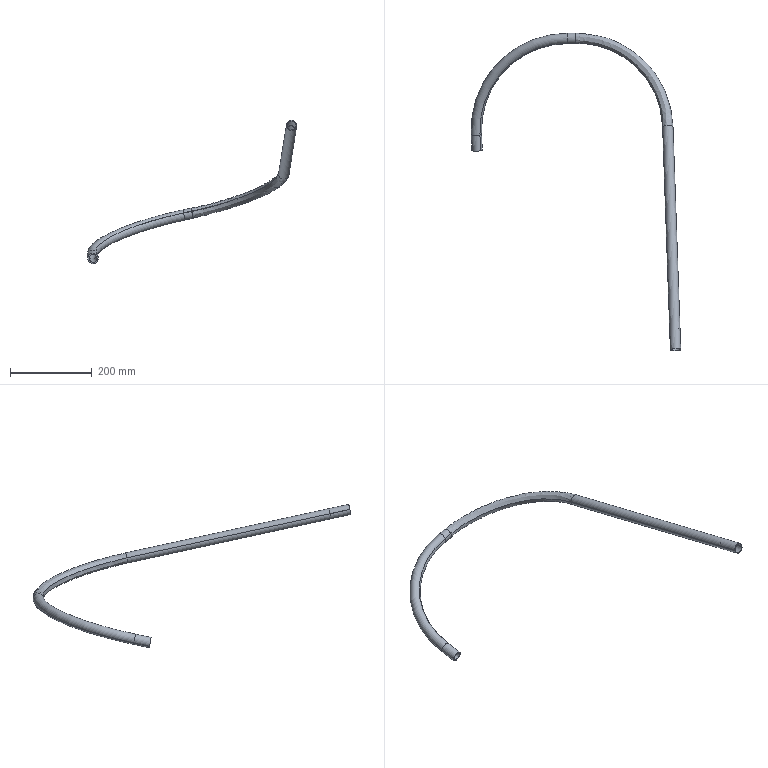Part | STEP file | 31E-01145WG10 | 1 solid | 25 faces | box 512.979 x 777.537 x 350.463 mm | volume 265200 mm3 | cylinder 14 | spline 4 | torus 4 | plane 3 | commonest cylinder face diameters 19.8 x6 25.4 x6 22.2 x2
STEP:
#1=CARTESIAN_POINT('',(-236.061,795.935,-46.108));
#2=VERTEX_POINT('',#1);
#3=CARTESIAN_POINT('',(-20.914,588.327,46.013));
#4=VERTEX_POINT('',#3);
#5=CARTESIAN_POINT('',(-20.914,588.327,46.013));
#6=CARTESIAN_POINT('',(-21.694,610.725,41.15));
#7=CARTESIAN_POINT('',(-25.248,632.89,35.656));
#8=CARTESIAN_POINT('',(-31.561,654.356,29.632));
#9=CARTESIAN_POINT('',(-49.455,695.005,16.849));
#10=CARTESIAN_POINT('',(-76.953,729.545,3.191));
#11=CARTESIAN_POINT('',(-92.871,744.902,-3.704));
#12=CARTESIAN_POINT('',(-128.381,771.151,-17.324));
#13=CARTESIAN_POINT('',(-169.661,787.598,-29.994));
#14=CARTESIAN_POINT('',(-191.348,793.153,-35.944));
#15=CARTESIAN_POINT('',(-213.636,795.932,-41.348));
#16=CARTESIAN_POINT('',(-236.061,795.935,-46.108));
#17=(BOUNDED_CURVE()B_SPLINE_CURVE(5,(#5,#6,#7,#8,#9,#10,#11,#12,#13,#14,#15,#16),.UNSPECIFIED.,.F.,.U.)B_SPLINE_CURVE_WITH_KNOTS((6,3,3,6),(0.,119.553,239.105,358.658),.UNSPECIFIED.)CURVE()GEOMETRIC_REPRESENTATION_ITEM()RATIONAL_B_SPLINE_CURVE((1.,1.,1.,1.,1.,1.,1.,1.,1.,1.,1.,1.))REPRESENTATION_ITEM(''));
#18=EDGE_CURVE('',#2,#4,#17,.F.);
#19=ORIENTED_EDGE('',*,*,#18,.F.);
#20=CARTESIAN_POINT('',(-234.406,814.065,-53.893));
#21=VERTEX_POINT('',#20);
#22=CARTESIAN_POINT('',(-236.061,795.935,-46.108));
#23=CARTESIAN_POINT('',(-237.946,799.915,-37.241));
#24=CARTESIAN_POINT('',(-238.061,810.969,-36.7));
#25=CARTESIAN_POINT('',(-236.291,818.044,-45.026));
#26=CARTESIAN_POINT('',(-234.406,814.065,-53.893));
#27=(BOUNDED_CURVE()B_SPLINE_CURVE(4,(#22,#23,#24,#25,#26),.UNSPECIFIED.,.F.,.U.)B_SPLINE_CURVE_WITH_KNOTS((5,5),(31.029,62.13),.UNSPECIFIED.)CURVE()GEOMETRIC_REPRESENTATION_ITEM()RATIONAL_B_SPLINE_CURVE((1.,0.7071,0.6667,0.7071,1.))REPRESENTATION_ITEM(''));
#28=EDGE_CURVE('',#2,#21,#27,.T.);
#29=ORIENTED_EDGE('',*,*,#28,.T.);
#30=CARTESIAN_POINT('',(-1.126,589.015,46.013));
#31=VERTEX_POINT('',#30);
#32=CARTESIAN_POINT('',(-1.126,589.015,46.013));
#33=CARTESIAN_POINT('',(-1.971,613.287,40.728));
#34=CARTESIAN_POINT('',(-5.823,637.306,34.765));
#35=CARTESIAN_POINT('',(-12.665,660.572,28.234));
#36=CARTESIAN_POINT('',(-32.061,704.635,14.377));
#37=CARTESIAN_POINT('',(-61.872,742.083,-0.4222));
#38=CARTESIAN_POINT('',(-79.13,758.735,-7.894));
#39=CARTESIAN_POINT('',(-117.632,787.197,-22.653));
#40=CARTESIAN_POINT('',(-162.396,805.033,-36.393));
#41=CARTESIAN_POINT('',(-185.915,811.057,-42.848));
#42=CARTESIAN_POINT('',(-210.087,814.068,-48.717));
#43=CARTESIAN_POINT('',(-234.406,814.065,-53.893));
#44=(BOUNDED_CURVE()B_SPLINE_CURVE(5,(#32,#33,#34,#35,#36,#37,#38,#39,#40,#41,#42,#43),.UNSPECIFIED.,.F.,.U.)B_SPLINE_CURVE_WITH_KNOTS((6,3,3,6),(0.,119.553,239.105,358.658),.UNSPECIFIED.)CURVE()GEOMETRIC_REPRESENTATION_ITEM()RATIONAL_B_SPLINE_CURVE((1.,1.,1.,1.,1.,1.,1.,1.,1.,1.,1.,1.))REPRESENTATION_ITEM(''));
#45=EDGE_CURVE('',#21,#31,#44,.F.);
#46=ORIENTED_EDGE('',*,*,#45,.T.);
#47=CARTESIAN_POINT('',(-20.914,588.327,46.013));
#48=CARTESIAN_POINT('',(-20.987,590.428,55.687));
#49=CARTESIAN_POINT('',(-11.13,591.823,60.524));
#50=CARTESIAN_POINT('',(-1.199,591.116,55.687));
#51=CARTESIAN_POINT('',(-1.126,589.015,46.013));
#52=(BOUNDED_CURVE()B_SPLINE_CURVE(4,(#47,#48,#49,#50,#51),.UNSPECIFIED.,.F.,.U.)B_SPLINE_CURVE_WITH_KNOTS((5,5),(31.029,62.13),.UNSPECIFIED.)CURVE()GEOMETRIC_REPRESENTATION_ITEM()RATIONAL_B_SPLINE_CURVE((1.,0.7071,0.6667,0.7071,1.))REPRESENTATION_ITEM(''));
#53=EDGE_CURVE('',#4,#31,#52,.T.);
#54=ORIENTED_EDGE('',*,*,#53,.F.);
#55=EDGE_LOOP('',(#19,#29,#46,#54));
#56=FACE_OUTER_BOUND('',#55,.T.);
#57=CARTESIAN_POINT('',(-20.914,588.327,46.013));
#58=CARTESIAN_POINT('',(-20.987,590.428,55.687));
#59=CARTESIAN_POINT('',(-11.13,591.823,60.524));
#60=CARTESIAN_POINT('',(-1.199,591.116,55.687));
#61=CARTESIAN_POINT('',(-1.126,589.015,46.013));
#62=CARTESIAN_POINT('',(-21.694,610.725,41.15));
#63=CARTESIAN_POINT('',(-21.767,613.043,50.777));
#64=CARTESIAN_POINT('',(-11.943,615.483,55.379));
#65=CARTESIAN_POINT('',(-2.044,615.605,50.355));
#66=CARTESIAN_POINT('',(-1.971,613.287,40.728));
#67=CARTESIAN_POINT('',(-25.248,632.89,35.656));
#68=CARTESIAN_POINT('',(-25.352,635.425,45.229));
#69=CARTESIAN_POINT('',(-15.691,638.9,49.571));
#70=CARTESIAN_POINT('',(-5.927,639.841,44.339));
#71=CARTESIAN_POINT('',(-5.823,637.306,34.765));
#72=CARTESIAN_POINT('',(-31.561,654.356,29.632));
#73=CARTESIAN_POINT('',(-31.725,657.093,39.148));
#74=CARTESIAN_POINT('',(-22.359,661.57,43.207));
#75=CARTESIAN_POINT('',(-12.829,663.309,37.75));
#76=CARTESIAN_POINT('',(-12.665,660.572,28.234));
#77=CARTESIAN_POINT('',(-49.455,695.005,16.849));
#78=CARTESIAN_POINT('',(-49.785,698.116,26.247));
#79=CARTESIAN_POINT('',(-41.252,704.486,29.711));
#80=CARTESIAN_POINT('',(-32.391,707.746,23.776));
#81=CARTESIAN_POINT('',(-32.061,704.635,14.377));
#82=CARTESIAN_POINT('',(-76.953,729.545,3.191));
#83=CARTESIAN_POINT('',(-77.53,732.959,12.469));
#84=CARTESIAN_POINT('',(-70.277,740.935,15.302));
#85=CARTESIAN_POINT('',(-62.449,745.497,8.856));
#86=CARTESIAN_POINT('',(-61.872,742.083,-0.4222));
#87=CARTESIAN_POINT('',(-92.871,744.902,-3.704));
#88=CARTESIAN_POINT('',(-93.588,748.449,5.514));
#89=CARTESIAN_POINT('',(-87.076,757.138,8.028));
#90=CARTESIAN_POINT('',(-79.847,762.281,1.325));
#91=CARTESIAN_POINT('',(-79.13,758.735,-7.894));
#92=CARTESIAN_POINT('',(-128.381,771.151,-17.324));
#93=CARTESIAN_POINT('',(-129.406,774.919,-8.221));
#94=CARTESIAN_POINT('',(-124.544,784.827,-6.335));
#95=CARTESIAN_POINT('',(-118.657,790.966,-13.551));
#96=CARTESIAN_POINT('',(-117.632,787.197,-22.653));
#97=CARTESIAN_POINT('',(-169.661,787.598,-29.994));
#98=CARTESIAN_POINT('',(-171.028,791.501,-20.997));
#99=CARTESIAN_POINT('',(-168.078,802.171,-19.697));
#100=CARTESIAN_POINT('',(-163.762,808.937,-27.395));
#101=CARTESIAN_POINT('',(-162.396,805.033,-36.393));
#102=CARTESIAN_POINT('',(-191.348,793.153,-35.944));
#103=CARTESIAN_POINT('',(-192.888,797.101,-26.994));
#104=CARTESIAN_POINT('',(-190.941,808.027,-25.971));
#105=CARTESIAN_POINT('',(-187.454,815.005,-33.898));
#106=CARTESIAN_POINT('',(-185.915,811.057,-42.848));
#107=CARTESIAN_POINT('',(-213.636,795.932,-41.348));
#108=CARTESIAN_POINT('',(-215.347,799.905,-32.441));
#109=CARTESIAN_POINT('',(-214.428,810.96,-31.672));
#110=CARTESIAN_POINT('',(-211.798,818.041,-39.81));
#111=CARTESIAN_POINT('',(-210.087,814.068,-48.717));
#112=CARTESIAN_POINT('',(-236.061,795.935,-46.108));
#113=CARTESIAN_POINT('',(-237.946,799.915,-37.241));
#114=CARTESIAN_POINT('',(-238.061,810.969,-36.7));
#115=CARTESIAN_POINT('',(-236.291,818.044,-45.026));
#116=CARTESIAN_POINT('',(-234.406,814.065,-53.893));
#117=(BOUNDED_SURFACE()B_SPLINE_SURFACE(5,4,((#57,#58,#59,#60,#61),(#62,#63,#64,#65,#66),(#67,#68,#69,#70,#71),(#72,#73,#74,#75,#76),(#77,#78,#79,#80,#81),(#82,#83,#84,#85,#86),(#87,#88,#89,#90,#91),(#92,#93,#94,#95,#96),(#97,#98,#99,#100,#101),(#102,#103,#104,#105,#106),(#107,#108,#109,#110,#111),(#112,#113,#114,#115,#116)),.UNSPECIFIED.,.F.,.F.,.U.)B_SPLINE_SURFACE_WITH_KNOTS((6,3,3,6),(5,5),(0.,119.553,239.105,358.658),(31.029,62.13),.UNSPECIFIED.)GEOMETRIC_REPRESENTATION_ITEM()RATIONAL_B_SPLINE_SURFACE(((1.,0.7071,0.6667,0.7071,1.),(1.,0.7071,0.6667,0.7071,1.),(1.,0.7071,0.6667,0.7071,1.),(1.,0.7071,0.6667,0.7071,1.),(1.,0.7071,0.6667,0.7071,1.),(1.,0.7071,0.6667,0.7071,1.),(1.,0.7071,0.6667,0.7071,1.),(1.,0.7071,0.6667,0.7071,1.),(1.,0.7071,0.6667,0.7071,1.),(1.,0.7071,0.6667,0.7071,1.),(1.,0.7071,0.6667,0.7071,1.),(1.,0.7071,0.6667,0.7071,1.)))REPRESENTATION_ITEM('')SURFACE());
#118=ADVANCED_FACE('',(#56),#117,.T.);
#119=ORIENTED_EDGE('',*,*,#45,.F.);
#120=CARTESIAN_POINT('',(-234.406,814.065,-53.893));
#121=CARTESIAN_POINT('',(-232.521,810.085,-62.76));
#122=CARTESIAN_POINT('',(-232.406,799.031,-63.301));
#123=CARTESIAN_POINT('',(-234.176,791.956,-54.975));
#124=CARTESIAN_POINT('',(-236.061,795.935,-46.108));
#125=(BOUNDED_CURVE()B_SPLINE_CURVE(4,(#120,#121,#122,#123,#124),.UNSPECIFIED.,.F.,.U.)B_SPLINE_CURVE_WITH_KNOTS((5,5),(62.13,93.232),.UNSPECIFIED.)CURVE()GEOMETRIC_REPRESENTATION_ITEM()RATIONAL_B_SPLINE_CURVE((1.,0.7071,0.6667,0.7071,1.))REPRESENTATION_ITEM(''));
#126=EDGE_CURVE('',#21,#2,#125,.T.);
#127=ORIENTED_EDGE('',*,*,#126,.T.);
#128=ORIENTED_EDGE('',*,*,#18,.T.);
#129=CARTESIAN_POINT('',(-1.126,589.015,46.013));
#130=CARTESIAN_POINT('',(-1.053,586.914,36.338));
#131=CARTESIAN_POINT('',(-10.91,585.52,31.501));
#132=CARTESIAN_POINT('',(-20.841,586.226,36.338));
#133=CARTESIAN_POINT('',(-20.914,588.327,46.013));
#134=(BOUNDED_CURVE()B_SPLINE_CURVE(4,(#129,#130,#131,#132,#133),.UNSPECIFIED.,.F.,.U.)B_SPLINE_CURVE_WITH_KNOTS((5,5),(62.13,93.232),.UNSPECIFIED.)CURVE()GEOMETRIC_REPRESENTATION_ITEM()RATIONAL_B_SPLINE_CURVE((1.,0.7071,0.6667,0.7071,1.))REPRESENTATION_ITEM(''));
#135=EDGE_CURVE('',#31,#4,#134,.T.);
#136=ORIENTED_EDGE('',*,*,#135,.F.);
#137=EDGE_LOOP('',(#119,#127,#128,#136));
#138=FACE_OUTER_BOUND('',#137,.T.);
#139=CARTESIAN_POINT('',(-1.126,589.015,46.013));
#140=CARTESIAN_POINT('',(-1.053,586.914,36.338));
#141=CARTESIAN_POINT('',(-10.91,585.52,31.501));
#142=CARTESIAN_POINT('',(-20.841,586.226,36.338));
#143=CARTESIAN_POINT('',(-20.914,588.327,46.013));
#144=CARTESIAN_POINT('',(-1.971,613.287,40.728));
#145=CARTESIAN_POINT('',(-1.897,610.969,31.101));
#146=CARTESIAN_POINT('',(-11.722,608.529,26.498));
#147=CARTESIAN_POINT('',(-21.62,608.407,31.522));
#148=CARTESIAN_POINT('',(-21.694,610.725,41.15));
#149=CARTESIAN_POINT('',(-5.823,637.306,34.765));
#150=CARTESIAN_POINT('',(-5.719,634.772,25.192));
#151=CARTESIAN_POINT('',(-15.38,631.297,20.85));
#152=CARTESIAN_POINT('',(-25.144,630.356,26.082));
#153=CARTESIAN_POINT('',(-25.248,632.89,35.656));
#154=CARTESIAN_POINT('',(-12.665,660.572,28.234));
#155=CARTESIAN_POINT('',(-12.502,657.834,18.718));
#156=CARTESIAN_POINT('',(-21.868,653.358,14.659));
#157=CARTESIAN_POINT('',(-31.398,651.619,20.116));
#158=CARTESIAN_POINT('',(-31.561,654.356,29.632));
#159=CARTESIAN_POINT('',(-32.061,704.635,14.377));
#160=CARTESIAN_POINT('',(-31.732,701.524,4.979));
#161=CARTESIAN_POINT('',(-40.265,695.154,1.515));
#162=CARTESIAN_POINT('',(-49.126,691.894,7.45));
#163=CARTESIAN_POINT('',(-49.455,695.005,16.849));
#164=CARTESIAN_POINT('',(-61.872,742.083,-0.4222));
#165=CARTESIAN_POINT('',(-61.296,738.669,-9.7));
#166=CARTESIAN_POINT('',(-68.548,730.693,-12.533));
#167=CARTESIAN_POINT('',(-76.377,726.131,-6.087));
#168=CARTESIAN_POINT('',(-76.953,729.545,3.191));
#169=CARTESIAN_POINT('',(-79.13,758.735,-7.894));
#170=CARTESIAN_POINT('',(-78.413,755.188,-17.112));
#171=CARTESIAN_POINT('',(-84.925,746.499,-19.627));
#172=CARTESIAN_POINT('',(-92.154,741.356,-12.923));
#173=CARTESIAN_POINT('',(-92.871,744.902,-3.704));
#174=CARTESIAN_POINT('',(-117.632,787.197,-22.653));
#175=CARTESIAN_POINT('',(-116.607,783.429,-31.756));
#176=CARTESIAN_POINT('',(-121.468,773.521,-33.642));
#177=CARTESIAN_POINT('',(-127.356,767.382,-26.426));
#178=CARTESIAN_POINT('',(-128.381,771.151,-17.324));
#179=CARTESIAN_POINT('',(-162.396,805.033,-36.393));
#180=CARTESIAN_POINT('',(-161.029,801.13,-45.391));
#181=CARTESIAN_POINT('',(-163.979,790.461,-46.691));
#182=CARTESIAN_POINT('',(-168.295,783.695,-38.992));
#183=CARTESIAN_POINT('',(-169.661,787.598,-29.994));
#184=CARTESIAN_POINT('',(-185.915,811.057,-42.848));
#185=CARTESIAN_POINT('',(-184.375,807.11,-51.798));
#186=CARTESIAN_POINT('',(-186.321,796.184,-52.821));
#187=CARTESIAN_POINT('',(-189.808,789.206,-44.894));
#188=CARTESIAN_POINT('',(-191.348,793.153,-35.944));
#189=CARTESIAN_POINT('',(-210.087,814.068,-48.717));
#190=CARTESIAN_POINT('',(-208.376,810.095,-57.624));
#191=CARTESIAN_POINT('',(-209.295,799.04,-58.393));
#192=CARTESIAN_POINT('',(-211.925,791.959,-50.255));
#193=CARTESIAN_POINT('',(-213.636,795.932,-41.348));
#194=CARTESIAN_POINT('',(-234.406,814.065,-53.893));
#195=CARTESIAN_POINT('',(-232.521,810.085,-62.76));
#196=CARTESIAN_POINT('',(-232.406,799.031,-63.301));
#197=CARTESIAN_POINT('',(-234.176,791.956,-54.975));
#198=CARTESIAN_POINT('',(-236.061,795.935,-46.108));
#199=(BOUNDED_SURFACE()B_SPLINE_SURFACE(5,4,((#139,#140,#141,#142,#143),(#144,#145,#146,#147,#148),(#149,#150,#151,#152,#153),(#154,#155,#156,#157,#158),(#159,#160,#161,#162,#163),(#164,#165,#166,#167,#168),(#169,#170,#171,#172,#173),(#174,#175,#176,#177,#178),(#179,#180,#181,#182,#183),(#184,#185,#186,#187,#188),(#189,#190,#191,#192,#193),(#194,#195,#196,#197,#198)),.UNSPECIFIED.,.F.,.F.,.U.)B_SPLINE_SURFACE_WITH_KNOTS((6,3,3,6),(5,5),(0.,119.553,239.105,358.658),(62.13,93.232),.UNSPECIFIED.)GEOMETRIC_REPRESENTATION_ITEM()RATIONAL_B_SPLINE_SURFACE(((1.,0.7071,0.6667,0.7071,1.),(1.,0.7071,0.6667,0.7071,1.),(1.,0.7071,0.6667,0.7071,1.),(1.,0.7071,0.6667,0.7071,1.),(1.,0.7071,0.6667,0.7071,1.),(1.,0.7071,0.6667,0.7071,1.),(1.,0.7071,0.6667,0.7071,1.),(1.,0.7071,0.6667,0.7071,1.),(1.,0.7071,0.6667,0.7071,1.),(1.,0.7071,0.6667,0.7071,1.),(1.,0.7071,0.6667,0.7071,1.),(1.,0.7071,0.6667,0.7071,1.)))REPRESENTATION_ITEM('')SURFACE());
#200=ADVANCED_FACE('',(#138),#199,.T.);
#201=CARTESIAN_POINT('',(20.666,43.336,164.685));
#202=VERTEX_POINT('',#201);
#203=CARTESIAN_POINT('',(1.672,589.113,46.013));
#204=VERTEX_POINT('',#203);
#205=CARTESIAN_POINT('',(11.169,316.224,105.349));
#206=DIRECTION('',(-0.03399,0.9766,-0.2123));
#207=VECTOR('',#206,1.);
#208=LINE('',#205,#207);
#209=EDGE_CURVE('',#202,#204,#208,.T.);
#210=ORIENTED_EDGE('',*,*,#209,.F.);
#211=CARTESIAN_POINT('',(-4.719,42.452,164.685));
#212=VERTEX_POINT('',#211);
#213=CARTESIAN_POINT('',(7.974,42.894,164.685));
#214=DIRECTION('',(-0.03399,0.9766,-0.2123));
#215=AXIS2_PLACEMENT_3D('',#213,#214,$);
#216=CIRCLE('',#215,12.7);
#217=EDGE_CURVE('',#202,#212,#216,.T.);
#218=ORIENTED_EDGE('',*,*,#217,.T.);
#219=CARTESIAN_POINT('',(-23.712,588.229,46.013));
#220=VERTEX_POINT('',#219);
#221=CARTESIAN_POINT('',(-14.215,315.341,105.349));
#222=DIRECTION('',(-0.03399,0.9766,-0.2123));
#223=VECTOR('',#222,1.);
#224=LINE('',#221,#223);
#225=EDGE_CURVE('',#212,#220,#224,.T.);
#226=ORIENTED_EDGE('',*,*,#225,.T.);
#227=CARTESIAN_POINT('',(-11.02,588.671,46.013));
#228=DIRECTION('',(-0.03399,0.9766,-0.2123));
#229=AXIS2_PLACEMENT_3D('',#227,#228,$);
#230=CIRCLE('',#229,12.7);
#231=EDGE_CURVE('',#204,#220,#230,.T.);
#232=ORIENTED_EDGE('',*,*,#231,.F.);
#233=EDGE_LOOP('',(#210,#218,#226,#232));
#234=FACE_OUTER_BOUND('',#233,.T.);
#235=CARTESIAN_POINT('',(-1.523,315.782,105.349));
#236=DIRECTION('',(-0.03399,0.9766,-0.2123));
#237=DIRECTION('',(0.9994,0.03478,0.));
#238=AXIS2_PLACEMENT_3D('',#235,#236,#237);
#239=CYLINDRICAL_SURFACE('',#238,12.7);
#240=ADVANCED_FACE('',(#234),#239,.T.);
#241=ORIENTED_EDGE('',*,*,#225,.F.);
#242=CARTESIAN_POINT('',(7.974,42.894,164.685));
#243=DIRECTION('',(-0.03399,0.9766,-0.2123));
#244=AXIS2_PLACEMENT_3D('',#242,#243,$);
#245=CIRCLE('',#244,12.7);
#246=EDGE_CURVE('',#212,#202,#245,.T.);
#247=ORIENTED_EDGE('',*,*,#246,.T.);
#248=ORIENTED_EDGE('',*,*,#209,.T.);
#249=CARTESIAN_POINT('',(-11.02,588.671,46.013));
#250=DIRECTION('',(-0.03399,0.9766,-0.2123));
#251=AXIS2_PLACEMENT_3D('',#249,#250,$);
#252=CIRCLE('',#251,12.7);
#253=EDGE_CURVE('',#220,#204,#252,.T.);
#254=ORIENTED_EDGE('',*,*,#253,.F.);
#255=EDGE_LOOP('',(#241,#247,#248,#254));
#256=FACE_OUTER_BOUND('',#255,.T.);
#257=CARTESIAN_POINT('',(-1.523,315.782,105.349));
#258=DIRECTION('',(-0.03399,0.9766,-0.2123));
#259=DIRECTION('',(-0.9994,-0.03478,0.));
#260=AXIS2_PLACEMENT_3D('',#257,#258,#259);
#261=CYLINDRICAL_SURFACE('',#260,12.7);
#262=ADVANCED_FACE('',(#256),#261,.T.);
#263=CARTESIAN_POINT('',(-255.83,795.935,-50.31));
#264=VERTEX_POINT('',#263);
#265=CARTESIAN_POINT('',(-254.176,814.065,-58.095));
#266=VERTEX_POINT('',#265);
#267=CARTESIAN_POINT('',(-255.003,805.,-54.203));
#268=DIRECTION('',(-0.9781,0.,-0.2079));
#269=AXIS2_PLACEMENT_3D('',#267,#268,$);
#270=CIRCLE('',#269,9.9);
#271=EDGE_CURVE('',#264,#266,#270,.T.);
#272=ORIENTED_EDGE('',*,*,#271,.T.);
#273=CARTESIAN_POINT('',(-244.291,814.065,-55.994));
#274=DIRECTION('',(-0.9781,0.,-0.2079));
#275=VECTOR('',#274,1.);
#276=LINE('',#273,#275);
#277=EDGE_CURVE('',#21,#266,#276,.T.);
#278=ORIENTED_EDGE('',*,*,#277,.F.);
#279=ORIENTED_EDGE('',*,*,#28,.F.);
#280=CARTESIAN_POINT('',(-245.946,795.935,-48.209));
#281=DIRECTION('',(-0.9781,0.,-0.2079));
#282=VECTOR('',#281,1.);
#283=LINE('',#280,#282);
#284=EDGE_CURVE('',#2,#264,#283,.T.);
#285=ORIENTED_EDGE('',*,*,#284,.T.);
#286=EDGE_LOOP('',(#272,#278,#279,#285));
#287=FACE_OUTER_BOUND('',#286,.T.);
#288=CARTESIAN_POINT('',(-245.118,805.,-52.101));
#289=DIRECTION('',(-0.9781,0.,-0.2079));
#290=DIRECTION('',(-0.08357,-0.9157,0.3932));
#291=AXIS2_PLACEMENT_3D('',#288,#289,#290);
#292=CYLINDRICAL_SURFACE('',#291,9.9);
#293=ADVANCED_FACE('',(#287),#292,.F.);
#294=CARTESIAN_POINT('',(-255.003,805.,-54.203));
#295=DIRECTION('',(-0.9781,0.,-0.2079));
#296=AXIS2_PLACEMENT_3D('',#294,#295,$);
#297=CIRCLE('',#296,9.9);
#298=EDGE_CURVE('',#266,#264,#297,.T.);
#299=ORIENTED_EDGE('',*,*,#298,.T.);
#300=ORIENTED_EDGE('',*,*,#284,.F.);
#301=ORIENTED_EDGE('',*,*,#126,.F.);
#302=ORIENTED_EDGE('',*,*,#277,.T.);
#303=EDGE_LOOP('',(#299,#300,#301,#302));
#304=FACE_OUTER_BOUND('',#303,.T.);
#305=CARTESIAN_POINT('',(-245.118,805.,-52.101));
#306=DIRECTION('',(-0.9781,0.,-0.2079));
#307=DIRECTION('',(0.08357,0.9157,-0.3932));
#308=AXIS2_PLACEMENT_3D('',#305,#306,#307);
#309=CYLINDRICAL_SURFACE('',#308,9.9);
#310=ADVANCED_FACE('',(#304),#309,.F.);
#311=ORIENTED_EDGE('',*,*,#231,.T.);
#312=CARTESIAN_POINT('',(-236.295,793.371,-45.007));
#313=VERTEX_POINT('',#312);
#314=CARTESIAN_POINT('',(-23.712,588.229,46.013));
#315=CARTESIAN_POINT('',(-24.483,610.363,41.209));
#316=CARTESIAN_POINT('',(-27.995,632.266,35.782));
#317=CARTESIAN_POINT('',(-34.234,653.477,29.83));
#318=CARTESIAN_POINT('',(-51.915,693.644,17.198));
#319=CARTESIAN_POINT('',(-79.086,727.772,3.702));
#320=CARTESIAN_POINT('',(-94.814,742.946,-3.112));
#321=CARTESIAN_POINT('',(-129.901,768.881,-16.57));
#322=CARTESIAN_POINT('',(-170.689,785.133,-29.09));
#323=CARTESIAN_POINT('',(-192.116,790.621,-34.968));
#324=CARTESIAN_POINT('',(-214.138,793.368,-40.306));
#325=CARTESIAN_POINT('',(-236.295,793.371,-45.007));
#326=(BOUNDED_CURVE()B_SPLINE_CURVE(5,(#314,#315,#316,#317,#318,#319,#320,#321,#322,#323,#324,#325),.UNSPECIFIED.,.F.,.U.)B_SPLINE_CURVE_WITH_KNOTS((6,3,3,6),(0.,119.604,239.209,358.815),.UNSPECIFIED.)CURVE()GEOMETRIC_REPRESENTATION_ITEM()RATIONAL_B_SPLINE_CURVE((1.,1.,1.,1.,1.,1.,1.,1.,1.,1.,1.,1.))REPRESENTATION_ITEM(''));
#327=EDGE_CURVE('',#313,#220,#326,.F.);
#328=ORIENTED_EDGE('',*,*,#327,.F.);
#329=CARTESIAN_POINT('',(-234.172,816.629,-54.994));
#330=VERTEX_POINT('',#329);
#331=CARTESIAN_POINT('',(-234.172,816.629,-54.994));
#332=CARTESIAN_POINT('',(-231.754,811.524,-66.369));
#333=CARTESIAN_POINT('',(-231.607,797.342,-67.062));
#334=CARTESIAN_POINT('',(-233.877,788.266,-56.382));
#335=CARTESIAN_POINT('',(-236.295,793.371,-45.007));
#336=(BOUNDED_CURVE()B_SPLINE_CURVE(4,(#331,#332,#333,#334,#335),.UNSPECIFIED.,.F.,.U.)B_SPLINE_CURVE_WITH_KNOTS((5,5),(79.703,119.601),.UNSPECIFIED.)CURVE()GEOMETRIC_REPRESENTATION_ITEM()RATIONAL_B_SPLINE_CURVE((1.,0.7071,0.6667,0.7071,1.))REPRESENTATION_ITEM(''));
#337=EDGE_CURVE('',#330,#313,#336,.T.);
#338=ORIENTED_EDGE('',*,*,#337,.F.);
#339=CARTESIAN_POINT('',(1.672,589.113,46.013));
#340=CARTESIAN_POINT('',(0.8184,613.649,40.668));
#341=CARTESIAN_POINT('',(-3.076,637.93,34.64));
#342=CARTESIAN_POINT('',(-9.993,661.451,28.036));
#343=CARTESIAN_POINT('',(-29.602,705.997,14.028));
#344=CARTESIAN_POINT('',(-59.74,743.856,-0.9331));
#345=CARTESIAN_POINT('',(-77.187,760.691,-8.486));
#346=CARTESIAN_POINT('',(-116.112,789.467,-23.407));
#347=CARTESIAN_POINT('',(-161.368,807.499,-37.298));
#348=CARTESIAN_POINT('',(-185.146,813.589,-43.824));
#349=CARTESIAN_POINT('',(-209.585,816.632,-49.759));
#350=CARTESIAN_POINT('',(-234.172,816.629,-54.994));
#351=(BOUNDED_CURVE()B_SPLINE_CURVE(5,(#339,#340,#341,#342,#343,#344,#345,#346,#347,#348,#349,#350),.UNSPECIFIED.,.F.,.U.)B_SPLINE_CURVE_WITH_KNOTS((6,3,3,6),(0.,119.604,239.209,358.815),.UNSPECIFIED.)CURVE()GEOMETRIC_REPRESENTATION_ITEM()RATIONAL_B_SPLINE_CURVE((1.,1.,1.,1.,1.,1.,1.,1.,1.,1.,1.,1.))REPRESENTATION_ITEM(''));
#352=EDGE_CURVE('',#330,#204,#351,.F.);
#353=ORIENTED_EDGE('',*,*,#352,.T.);
#354=EDGE_LOOP('',(#311,#328,#338,#353));
#355=FACE_OUTER_BOUND('',#354,.T.);
#356=CARTESIAN_POINT('',(1.672,589.113,46.013));
#357=CARTESIAN_POINT('',(1.766,586.418,33.602));
#358=CARTESIAN_POINT('',(-10.879,584.628,27.397));
#359=CARTESIAN_POINT('',(-23.619,585.534,33.602));
#360=CARTESIAN_POINT('',(-23.712,588.229,46.013));
#361=CARTESIAN_POINT('',(0.8184,613.649,40.668));
#362=CARTESIAN_POINT('',(0.9129,610.676,28.318));
#363=CARTESIAN_POINT('',(-11.69,607.546,22.414));
#364=CARTESIAN_POINT('',(-24.388,607.389,28.859));
#365=CARTESIAN_POINT('',(-24.483,610.363,41.209));
#366=CARTESIAN_POINT('',(-3.076,637.93,34.64));
#367=CARTESIAN_POINT('',(-2.943,634.679,22.358));
#368=CARTESIAN_POINT('',(-15.336,630.221,16.789));
#369=CARTESIAN_POINT('',(-27.862,629.014,23.501));
#370=CARTESIAN_POINT('',(-27.995,632.266,35.782));
#371=CARTESIAN_POINT('',(-9.993,661.451,28.036));
#372=CARTESIAN_POINT('',(-9.783,657.939,15.828));
#373=CARTESIAN_POINT('',(-21.799,652.197,10.621));
#374=CARTESIAN_POINT('',(-34.024,649.966,17.622));
#375=CARTESIAN_POINT('',(-34.234,653.477,29.83));
#376=CARTESIAN_POINT('',(-29.602,705.997,14.028));
#377=CARTESIAN_POINT('',(-29.18,702.006,1.971));
#378=CARTESIAN_POINT('',(-40.125,693.834,-2.472));
#379=CARTESIAN_POINT('',(-51.493,689.653,5.141));
#380=CARTESIAN_POINT('',(-51.915,693.644,17.198));
#381=CARTESIAN_POINT('',(-59.74,743.856,-0.9331));
#382=CARTESIAN_POINT('',(-59.,739.477,-12.835));
#383=CARTESIAN_POINT('',(-68.303,729.245,-16.469));
#384=CARTESIAN_POINT('',(-78.346,723.393,-8.2));
#385=CARTESIAN_POINT('',(-79.086,727.772,3.702));
#386=CARTESIAN_POINT('',(-77.187,760.691,-8.486));
#387=CARTESIAN_POINT('',(-76.267,756.141,-20.312));
#388=CARTESIAN_POINT('',(-84.621,744.994,-23.537));
#389=CARTESIAN_POINT('',(-93.894,738.397,-14.937));
#390=CARTESIAN_POINT('',(-94.814,742.946,-3.112));
#391=CARTESIAN_POINT('',(-116.112,789.467,-23.407));
#392=CARTESIAN_POINT('',(-114.797,784.632,-35.084));
#393=CARTESIAN_POINT('',(-121.034,771.922,-37.503));
#394=CARTESIAN_POINT('',(-128.586,764.047,-28.246));
#395=CARTESIAN_POINT('',(-129.901,768.881,-16.57));
#396=CARTESIAN_POINT('',(-161.368,807.499,-37.298));
#397=CARTESIAN_POINT('',(-159.615,802.492,-48.841));
#398=CARTESIAN_POINT('',(-163.399,788.805,-50.508));
#399=CARTESIAN_POINT('',(-168.936,780.125,-40.632));
#400=CARTESIAN_POINT('',(-170.689,785.133,-29.09));
#401=CARTESIAN_POINT('',(-185.146,813.589,-43.824));
#402=CARTESIAN_POINT('',(-183.171,808.525,-55.306));
#403=CARTESIAN_POINT('',(-185.668,794.509,-56.618));
#404=CARTESIAN_POINT('',(-190.141,785.557,-46.449));
#405=CARTESIAN_POINT('',(-192.116,790.621,-34.968));
#406=CARTESIAN_POINT('',(-209.585,816.632,-49.759));
#407=CARTESIAN_POINT('',(-207.39,811.536,-61.185));
#408=CARTESIAN_POINT('',(-208.569,797.355,-62.171));
#409=CARTESIAN_POINT('',(-211.943,788.271,-51.731));
#410=CARTESIAN_POINT('',(-214.138,793.368,-40.306));
#411=CARTESIAN_POINT('',(-234.172,816.629,-54.994));
#412=CARTESIAN_POINT('',(-231.754,811.524,-66.369));
#413=CARTESIAN_POINT('',(-231.607,797.342,-67.062));
#414=CARTESIAN_POINT('',(-233.877,788.266,-56.382));
#415=CARTESIAN_POINT('',(-236.295,793.371,-45.007));
#416=(BOUNDED_SURFACE()B_SPLINE_SURFACE(5,4,((#356,#357,#358,#359,#360),(#361,#362,#363,#364,#365),(#366,#367,#368,#369,#370),(#371,#372,#373,#374,#375),(#376,#377,#378,#379,#380),(#381,#382,#383,#384,#385),(#386,#387,#388,#389,#390),(#391,#392,#393,#394,#395),(#396,#397,#398,#399,#400),(#401,#402,#403,#404,#405),(#406,#407,#408,#409,#410),(#411,#412,#413,#414,#415)),.UNSPECIFIED.,.F.,.F.,.U.)B_SPLINE_SURFACE_WITH_KNOTS((6,3,3,6),(5,5),(0.,119.604,239.209,358.815),(79.703,119.601),.UNSPECIFIED.)GEOMETRIC_REPRESENTATION_ITEM()RATIONAL_B_SPLINE_SURFACE(((1.,0.7071,0.6667,0.7071,1.),(1.,0.7071,0.6667,0.7071,1.),(1.,0.7071,0.6667,0.7071,1.),(1.,0.7071,0.6667,0.7071,1.),(1.,0.7071,0.6667,0.7071,1.),(1.,0.7071,0.6667,0.7071,1.),(1.,0.7071,0.6667,0.7071,1.),(1.,0.7071,0.6667,0.7071,1.),(1.,0.7071,0.6667,0.7071,1.),(1.,0.7071,0.6667,0.7071,1.),(1.,0.7071,0.6667,0.7071,1.),(1.,0.7071,0.6667,0.7071,1.)))REPRESENTATION_ITEM('')SURFACE());
#417=ADVANCED_FACE('',(#355),#416,.F.);
#418=ORIENTED_EDGE('',*,*,#253,.T.);
#419=ORIENTED_EDGE('',*,*,#352,.F.);
#420=CARTESIAN_POINT('',(-236.295,793.371,-45.007));
#421=CARTESIAN_POINT('',(-238.713,798.476,-33.632));
#422=CARTESIAN_POINT('',(-238.86,812.658,-32.938));
#423=CARTESIAN_POINT('',(-236.59,821.734,-43.619));
#424=CARTESIAN_POINT('',(-234.172,816.629,-54.994));
#425=(BOUNDED_CURVE()B_SPLINE_CURVE(4,(#420,#421,#422,#423,#424),.UNSPECIFIED.,.F.,.U.)B_SPLINE_CURVE_WITH_KNOTS((5,5),(39.804,79.703),.UNSPECIFIED.)CURVE()GEOMETRIC_REPRESENTATION_ITEM()RATIONAL_B_SPLINE_CURVE((1.,0.7071,0.6667,0.7071,1.))REPRESENTATION_ITEM(''));
#426=EDGE_CURVE('',#313,#330,#425,.T.);
#427=ORIENTED_EDGE('',*,*,#426,.F.);
#428=ORIENTED_EDGE('',*,*,#327,.T.);
#429=EDGE_LOOP('',(#418,#419,#427,#428));
#430=FACE_OUTER_BOUND('',#429,.T.);
#431=CARTESIAN_POINT('',(-23.712,588.229,46.013));
#432=CARTESIAN_POINT('',(-23.806,590.925,58.423));
#433=CARTESIAN_POINT('',(-11.161,592.714,64.628));
#434=CARTESIAN_POINT('',(1.579,591.808,58.423));
#435=CARTESIAN_POINT('',(1.672,589.113,46.013));
#436=CARTESIAN_POINT('',(-24.483,610.363,41.209));
#437=CARTESIAN_POINT('',(-24.577,613.336,53.559));
#438=CARTESIAN_POINT('',(-11.974,616.466,59.464));
#439=CARTESIAN_POINT('',(0.724,616.623,53.018));
#440=CARTESIAN_POINT('',(0.8184,613.649,40.668));
#441=CARTESIAN_POINT('',(-27.995,632.266,35.782));
#442=CARTESIAN_POINT('',(-28.128,635.517,48.063));
#443=CARTESIAN_POINT('',(-15.735,639.975,53.632));
#444=CARTESIAN_POINT('',(-3.209,641.182,46.921));
#445=CARTESIAN_POINT('',(-3.076,637.93,34.64));
#446=CARTESIAN_POINT('',(-34.234,653.477,29.83));
#447=CARTESIAN_POINT('',(-34.444,656.989,42.037));
#448=CARTESIAN_POINT('',(-22.428,662.732,47.244));
#449=CARTESIAN_POINT('',(-10.203,664.963,40.244));
#450=CARTESIAN_POINT('',(-9.993,661.451,28.036));
#451=CARTESIAN_POINT('',(-51.915,693.644,17.198));
#452=CARTESIAN_POINT('',(-52.338,697.634,29.255));
#453=CARTESIAN_POINT('',(-41.392,705.806,33.698));
#454=CARTESIAN_POINT('',(-30.024,709.987,26.084));
#455=CARTESIAN_POINT('',(-29.602,705.997,14.028));
#456=CARTESIAN_POINT('',(-79.086,727.772,3.702));
#457=CARTESIAN_POINT('',(-79.825,732.152,15.604));
#458=CARTESIAN_POINT('',(-70.522,742.384,19.238));
#459=CARTESIAN_POINT('',(-60.479,748.236,10.969));
#460=CARTESIAN_POINT('',(-59.74,743.856,-0.9331));
#461=CARTESIAN_POINT('',(-94.814,742.946,-3.112));
#462=CARTESIAN_POINT('',(-95.734,747.495,8.714));
#463=CARTESIAN_POINT('',(-87.38,758.642,11.939));
#464=CARTESIAN_POINT('',(-78.107,765.24,3.339));
#465=CARTESIAN_POINT('',(-77.187,760.691,-8.486));
#466=CARTESIAN_POINT('',(-129.901,768.881,-16.57));
#467=CARTESIAN_POINT('',(-131.216,773.716,-4.893));
#468=CARTESIAN_POINT('',(-124.979,786.426,-2.474));
#469=CARTESIAN_POINT('',(-117.427,794.301,-11.73));
#470=CARTESIAN_POINT('',(-116.112,789.467,-23.407));
#471=CARTESIAN_POINT('',(-170.689,785.133,-29.09));
#472=CARTESIAN_POINT('',(-172.442,790.14,-17.547));
#473=CARTESIAN_POINT('',(-168.658,803.827,-15.88));
#474=CARTESIAN_POINT('',(-163.121,812.506,-25.755));
#475=CARTESIAN_POINT('',(-161.368,807.499,-37.298));
#476=CARTESIAN_POINT('',(-192.116,790.621,-34.968));
#477=CARTESIAN_POINT('',(-194.092,795.685,-23.486));
#478=CARTESIAN_POINT('',(-191.594,809.701,-22.174));
#479=CARTESIAN_POINT('',(-187.122,818.653,-32.343));
#480=CARTESIAN_POINT('',(-185.146,813.589,-43.824));
#481=CARTESIAN_POINT('',(-214.138,793.368,-40.306));
#482=CARTESIAN_POINT('',(-216.332,798.464,-28.88));
#483=CARTESIAN_POINT('',(-215.154,812.645,-27.894));
#484=CARTESIAN_POINT('',(-211.78,821.729,-38.334));
#485=CARTESIAN_POINT('',(-209.585,816.632,-49.759));
#486=CARTESIAN_POINT('',(-236.295,793.371,-45.007));
#487=CARTESIAN_POINT('',(-238.713,798.476,-33.632));
#488=CARTESIAN_POINT('',(-238.86,812.658,-32.938));
#489=CARTESIAN_POINT('',(-236.59,821.734,-43.619));
#490=CARTESIAN_POINT('',(-234.172,816.629,-54.994));
#491=(BOUNDED_SURFACE()B_SPLINE_SURFACE(5,4,((#431,#432,#433,#434,#435),(#436,#437,#438,#439,#440),(#441,#442,#443,#444,#445),(#446,#447,#448,#449,#450),(#451,#452,#453,#454,#455),(#456,#457,#458,#459,#460),(#461,#462,#463,#464,#465),(#466,#467,#468,#469,#470),(#471,#472,#473,#474,#475),(#476,#477,#478,#479,#480),(#481,#482,#483,#484,#485),(#486,#487,#488,#489,#490)),.UNSPECIFIED.,.F.,.F.,.U.)B_SPLINE_SURFACE_WITH_KNOTS((6,3,3,6),(5,5),(0.,119.604,239.209,358.815),(39.804,79.703),.UNSPECIFIED.)GEOMETRIC_REPRESENTATION_ITEM()RATIONAL_B_SPLINE_SURFACE(((1.,0.7071,0.6667,0.7071,1.),(1.,0.7071,0.6667,0.7071,1.),(1.,0.7071,0.6667,0.7071,1.),(1.,0.7071,0.6667,0.7071,1.),(1.,0.7071,0.6667,0.7071,1.),(1.,0.7071,0.6667,0.7071,1.),(1.,0.7071,0.6667,0.7071,1.),(1.,0.7071,0.6667,0.7071,1.),(1.,0.7071,0.6667,0.7071,1.),(1.,0.7071,0.6667,0.7071,1.),(1.,0.7071,0.6667,0.7071,1.),(1.,0.7071,0.6667,0.7071,1.)))REPRESENTATION_ITEM('')SURFACE());
#492=ADVANCED_FACE('',(#430),#491,.F.);
#493=CARTESIAN_POINT('',(-472.695,569.043,-145.711));
#494=VERTEX_POINT('',#493);
#495=CARTESIAN_POINT('',(-486.073,571.446,-160.109));
#496=VERTEX_POINT('',#495);
#497=CARTESIAN_POINT('',(-479.384,570.245,-152.91));
#498=DIRECTION('',(-0.04323,0.9781,0.2034));
#499=AXIS2_PLACEMENT_3D('',#497,#498,$);
#500=CIRCLE('',#499,9.9);
#501=EDGE_CURVE('',#494,#496,#500,.F.);
#502=ORIENTED_EDGE('',*,*,#501,.T.);
#503=CARTESIAN_POINT('',(-243.454,571.446,-108.539));
#504=DIRECTION('',(-0.2034,-0.2079,0.9568));
#505=AXIS2_PLACEMENT_3D('',#503,#504,$);
#506=CIRCLE('',#505,248.039);
#507=EDGE_CURVE('',#266,#496,#506,.T.);
#508=ORIENTED_EDGE('',*,*,#507,.F.);
#509=ORIENTED_EDGE('',*,*,#271,.F.);
#510=CARTESIAN_POINT('',(-245.803,569.043,-97.483));
#511=DIRECTION('',(-0.2034,-0.2079,0.9568));
#512=AXIS2_PLACEMENT_3D('',#510,#511,$);
#513=CIRCLE('',#512,231.961);
#514=EDGE_CURVE('',#264,#494,#513,.T.);
#515=ORIENTED_EDGE('',*,*,#514,.T.);
#516=EDGE_LOOP('',(#502,#508,#509,#515));
#517=FACE_OUTER_BOUND('',#516,.T.);
#518=CARTESIAN_POINT('',(-244.629,570.245,-103.011));
#519=DIRECTION('',(-0.2034,-0.2079,0.9568));
#520=DIRECTION('',(-0.04323,0.9781,0.2034));
#521=AXIS2_PLACEMENT_3D('',#518,#519,#520);
#522=TOROIDAL_SURFACE('',#521,240.,9.9);
#523=ADVANCED_FACE('',(#517),#522,.F.);
#524=CARTESIAN_POINT('',(-479.384,570.245,-152.91));
#525=DIRECTION('',(-0.04323,0.9781,0.2034));
#526=AXIS2_PLACEMENT_3D('',#524,#525,$);
#527=CIRCLE('',#526,9.9);
#528=EDGE_CURVE('',#496,#494,#527,.F.);
#529=ORIENTED_EDGE('',*,*,#528,.T.);
#530=ORIENTED_EDGE('',*,*,#514,.F.);
#531=ORIENTED_EDGE('',*,*,#298,.F.);
#532=ORIENTED_EDGE('',*,*,#507,.T.);
#533=EDGE_LOOP('',(#529,#530,#531,#532));
#534=FACE_OUTER_BOUND('',#533,.T.);
#535=CARTESIAN_POINT('',(-244.629,570.245,-103.011));
#536=DIRECTION('',(-0.2034,-0.2079,0.9568));
#537=DIRECTION('',(-0.04323,0.9781,0.2034));
#538=AXIS2_PLACEMENT_3D('',#535,#536,#537);
#539=TOROIDAL_SURFACE('',#538,240.,9.9);
#540=ADVANCED_FACE('',(#534),#539,.F.);
#541=CARTESIAN_POINT('',(-253.942,816.629,-59.196));
#542=VERTEX_POINT('',#541);
#543=CARTESIAN_POINT('',(-244.057,816.629,-57.095));
#544=DIRECTION('',(-0.9781,0.,-0.2079));
#545=VECTOR('',#544,1.);
#546=LINE('',#543,#545);
#547=EDGE_CURVE('',#330,#542,#546,.T.);
#548=ORIENTED_EDGE('',*,*,#547,.F.);
#549=ORIENTED_EDGE('',*,*,#337,.T.);
#550=CARTESIAN_POINT('',(-256.064,793.371,-49.209));
#551=VERTEX_POINT('',#550);
#552=CARTESIAN_POINT('',(-246.18,793.371,-47.108));
#553=DIRECTION('',(-0.9781,0.,-0.2079));
#554=VECTOR('',#553,1.);
#555=LINE('',#552,#554);
#556=EDGE_CURVE('',#313,#551,#555,.T.);
#557=ORIENTED_EDGE('',*,*,#556,.T.);
#558=CARTESIAN_POINT('',(-255.003,805.,-54.203));
#559=DIRECTION('',(-0.9781,0.,-0.2079));
#560=AXIS2_PLACEMENT_3D('',#558,#559,$);
#561=CIRCLE('',#560,12.7);
#562=EDGE_CURVE('',#542,#551,#561,.T.);
#563=ORIENTED_EDGE('',*,*,#562,.F.);
#564=EDGE_LOOP('',(#548,#549,#557,#563));
#565=FACE_OUTER_BOUND('',#564,.T.);
#566=CARTESIAN_POINT('',(-245.118,805.,-52.101));
#567=DIRECTION('',(-0.9781,0.,-0.2079));
#568=DIRECTION('',(0.08357,0.9157,-0.3932));
#569=AXIS2_PLACEMENT_3D('',#566,#567,#568);
#570=CYLINDRICAL_SURFACE('',#569,12.7);
#571=ADVANCED_FACE('',(#565),#570,.T.);
#572=ORIENTED_EDGE('',*,*,#556,.F.);
#573=ORIENTED_EDGE('',*,*,#426,.T.);
#574=ORIENTED_EDGE('',*,*,#547,.T.);
#575=CARTESIAN_POINT('',(-255.003,805.,-54.203));
#576=DIRECTION('',(-0.9781,0.,-0.2079));
#577=AXIS2_PLACEMENT_3D('',#575,#576,$);
#578=CIRCLE('',#577,12.7);
#579=EDGE_CURVE('',#551,#542,#578,.T.);
#580=ORIENTED_EDGE('',*,*,#579,.F.);
#581=EDGE_LOOP('',(#572,#573,#574,#580));
#582=FACE_OUTER_BOUND('',#581,.T.);
#583=CARTESIAN_POINT('',(-245.118,805.,-52.101));
#584=DIRECTION('',(-0.9781,0.,-0.2079));
#585=DIRECTION('',(-0.08357,-0.9157,0.3932));
#586=AXIS2_PLACEMENT_3D('',#583,#584,#585);
#587=CYLINDRICAL_SURFACE('',#586,12.7);
#588=ADVANCED_FACE('',(#582),#587,.T.);
#589=CARTESIAN_POINT('',(-470.99,530.453,-153.734));
#590=VERTEX_POINT('',#589);
#591=CARTESIAN_POINT('',(-484.367,532.855,-168.132));
#592=VERTEX_POINT('',#591);
#593=CARTESIAN_POINT('',(-477.679,531.654,-160.933));
#594=DIRECTION('',(0.04323,-0.9781,-0.2034));
#595=AXIS2_PLACEMENT_3D('',#593,#594,$);
#596=CIRCLE('',#595,9.9);
#597=EDGE_CURVE('',#590,#592,#596,.T.);
#598=ORIENTED_EDGE('',*,*,#597,.T.);
#599=CARTESIAN_POINT('',(-485.22,552.151,-164.121));
#600=DIRECTION('',(0.04323,-0.9781,-0.2034));
#601=VECTOR('',#600,1.);
#602=LINE('',#599,#601);
#603=EDGE_CURVE('',#496,#592,#602,.T.);
#604=ORIENTED_EDGE('',*,*,#603,.F.);
#605=ORIENTED_EDGE('',*,*,#501,.F.);
#606=CARTESIAN_POINT('',(-471.842,549.748,-149.722));
#607=DIRECTION('',(0.04323,-0.9781,-0.2034));
#608=VECTOR('',#607,1.);
#609=LINE('',#606,#608);
#610=EDGE_CURVE('',#494,#590,#609,.T.);
#611=ORIENTED_EDGE('',*,*,#610,.T.);
#612=EDGE_LOOP('',(#598,#604,#605,#611));
#613=FACE_OUTER_BOUND('',#612,.T.);
#614=CARTESIAN_POINT('',(-478.531,550.949,-156.921));
#615=DIRECTION('',(0.04323,-0.9781,-0.2034));
#616=DIRECTION('',(0.6756,-0.1213,0.7272));
#617=AXIS2_PLACEMENT_3D('',#614,#615,#616);
#618=CYLINDRICAL_SURFACE('',#617,9.9);
#619=ADVANCED_FACE('',(#613),#618,.F.);
#620=CARTESIAN_POINT('',(-477.679,531.654,-160.933));
#621=DIRECTION('',(0.04323,-0.9781,-0.2034));
#622=AXIS2_PLACEMENT_3D('',#620,#621,$);
#623=CIRCLE('',#622,9.9);
#624=EDGE_CURVE('',#592,#590,#623,.T.);
#625=ORIENTED_EDGE('',*,*,#624,.T.);
#626=ORIENTED_EDGE('',*,*,#610,.F.);
#627=ORIENTED_EDGE('',*,*,#528,.F.);
#628=ORIENTED_EDGE('',*,*,#603,.T.);
#629=EDGE_LOOP('',(#625,#626,#627,#628));
#630=FACE_OUTER_BOUND('',#629,.T.);
#631=CARTESIAN_POINT('',(-478.531,550.949,-156.921));
#632=DIRECTION('',(0.04323,-0.9781,-0.2034));
#633=DIRECTION('',(-0.6756,0.1213,-0.7272));
#634=AXIS2_PLACEMENT_3D('',#631,#632,#633);
#635=CYLINDRICAL_SURFACE('',#634,9.9);
#636=ADVANCED_FACE('',(#630),#635,.F.);
#637=CARTESIAN_POINT('',(-487.965,571.785,-162.145));
#638=VERTEX_POINT('',#637);
#639=CARTESIAN_POINT('',(-243.121,571.785,-110.102));
#640=DIRECTION('',(-0.2034,-0.2079,0.9568));
#641=AXIS2_PLACEMENT_3D('',#639,#640,$);
#642=CIRCLE('',#641,250.313);
#643=EDGE_CURVE('',#542,#638,#642,.T.);
#644=ORIENTED_EDGE('',*,*,#643,.F.);
#645=ORIENTED_EDGE('',*,*,#562,.T.);
#646=CARTESIAN_POINT('',(-470.803,568.704,-143.675));
#647=VERTEX_POINT('',#646);
#648=CARTESIAN_POINT('',(-246.136,568.704,-95.92));
#649=DIRECTION('',(-0.2034,-0.2079,0.9568));
#650=AXIS2_PLACEMENT_3D('',#648,#649,$);
#651=CIRCLE('',#650,229.687);
#652=EDGE_CURVE('',#551,#647,#651,.T.);
#653=ORIENTED_EDGE('',*,*,#652,.T.);
#654=CARTESIAN_POINT('',(-479.384,570.245,-152.91));
#655=DIRECTION('',(-0.04323,0.9781,0.2034));
#656=AXIS2_PLACEMENT_3D('',#654,#655,$);
#657=CIRCLE('',#656,12.7);
#658=EDGE_CURVE('',#638,#647,#657,.F.);
#659=ORIENTED_EDGE('',*,*,#658,.F.);
#660=EDGE_LOOP('',(#644,#645,#653,#659));
#661=FACE_OUTER_BOUND('',#660,.T.);
#662=CARTESIAN_POINT('',(-244.629,570.245,-103.011));
#663=DIRECTION('',(-0.2034,-0.2079,0.9568));
#664=DIRECTION('',(-0.04323,0.9781,0.2034));
#665=AXIS2_PLACEMENT_3D('',#662,#663,#664);
#666=TOROIDAL_SURFACE('',#665,240.,12.7);
#667=ADVANCED_FACE('',(#661),#666,.T.);
#668=ORIENTED_EDGE('',*,*,#652,.F.);
#669=ORIENTED_EDGE('',*,*,#579,.T.);
#670=ORIENTED_EDGE('',*,*,#643,.T.);
#671=CARTESIAN_POINT('',(-479.384,570.245,-152.91));
#672=DIRECTION('',(-0.04323,0.9781,0.2034));
#673=AXIS2_PLACEMENT_3D('',#671,#672,$);
#674=CIRCLE('',#673,12.7);
#675=EDGE_CURVE('',#647,#638,#674,.F.);
#676=ORIENTED_EDGE('',*,*,#675,.F.);
#677=EDGE_LOOP('',(#668,#669,#670,#676));
#678=FACE_OUTER_BOUND('',#677,.T.);
#679=CARTESIAN_POINT('',(-244.629,570.245,-103.011));
#680=DIRECTION('',(-0.2034,-0.2079,0.9568));
#681=DIRECTION('',(-0.04323,0.9781,0.2034));
#682=AXIS2_PLACEMENT_3D('',#679,#680,#681);
#683=TOROIDAL_SURFACE('',#682,240.,12.7);
#684=ADVANCED_FACE('',(#678),#683,.T.);
#685=CARTESIAN_POINT('',(-486.259,533.195,-170.168));
#686=VERTEX_POINT('',#685);
#687=CARTESIAN_POINT('',(-469.098,530.113,-151.698));
#688=VERTEX_POINT('',#687);
#689=CARTESIAN_POINT('',(-477.679,531.654,-160.933));
#690=DIRECTION('',(-0.04323,0.9781,0.2034));
#691=AXIS2_PLACEMENT_3D('',#689,#690,$);
#692=CIRCLE('',#691,12.7);
#693=EDGE_CURVE('',#686,#688,#692,.T.);
#694=ORIENTED_EDGE('',*,*,#693,.F.);
#695=CARTESIAN_POINT('',(-477.679,531.654,-160.933));
#696=DIRECTION('',(-0.04323,0.9781,0.2034));
#697=AXIS2_PLACEMENT_3D('',#695,#696,$);
#698=CIRCLE('',#697,12.7);
#699=EDGE_CURVE('',#688,#686,#698,.T.);
#700=ORIENTED_EDGE('',*,*,#699,.F.);
#701=EDGE_LOOP('',(#694,#700));
#702=FACE_OUTER_BOUND('',#701,.T.);
#703=ORIENTED_EDGE('',*,*,#597,.F.);
#704=ORIENTED_EDGE('',*,*,#624,.F.);
#705=EDGE_LOOP('',(#703,#704));
#706=FACE_BOUND('',#705,.T.);
#707=CARTESIAN_POINT('',(-477.679,531.654,-160.933));
#708=DIRECTION('',(-0.04323,0.9781,0.2034));
#709=DIRECTION('',(0.2034,0.2079,-0.9568));
#710=AXIS2_PLACEMENT_3D('',#707,#708,#709);
#711=PLANE('',#710);
#712=ADVANCED_FACE('',(#702,#706),#711,.F.);
#713=CARTESIAN_POINT('',(-487.112,552.49,-166.157));
#714=DIRECTION('',(0.04323,-0.9781,-0.2034));
#715=VECTOR('',#714,1.);
#716=LINE('',#713,#715);
#717=EDGE_CURVE('',#638,#686,#716,.T.);
#718=ORIENTED_EDGE('',*,*,#717,.F.);
#719=ORIENTED_EDGE('',*,*,#658,.T.);
#720=CARTESIAN_POINT('',(-469.951,549.409,-147.686));
#721=DIRECTION('',(0.04323,-0.9781,-0.2034));
#722=VECTOR('',#721,1.);
#723=LINE('',#720,#722);
#724=EDGE_CURVE('',#647,#688,#723,.T.);
#725=ORIENTED_EDGE('',*,*,#724,.T.);
#726=ORIENTED_EDGE('',*,*,#699,.T.);
#727=EDGE_LOOP('',(#718,#719,#725,#726));
#728=FACE_OUTER_BOUND('',#727,.T.);
#729=CARTESIAN_POINT('',(-478.531,550.949,-156.921));
#730=DIRECTION('',(0.04323,-0.9781,-0.2034));
#731=DIRECTION('',(-0.6756,0.1213,-0.7272));
#732=AXIS2_PLACEMENT_3D('',#729,#730,#731);
#733=CYLINDRICAL_SURFACE('',#732,12.7);
#734=ADVANCED_FACE('',(#728),#733,.T.);
#735=ORIENTED_EDGE('',*,*,#724,.F.);
#736=ORIENTED_EDGE('',*,*,#675,.T.);
#737=ORIENTED_EDGE('',*,*,#717,.T.);
#738=ORIENTED_EDGE('',*,*,#693,.T.);
#739=EDGE_LOOP('',(#735,#736,#737,#738));
#740=FACE_OUTER_BOUND('',#739,.T.);
#741=CARTESIAN_POINT('',(-478.531,550.949,-156.921));
#742=DIRECTION('',(0.04323,-0.9781,-0.2034));
#743=DIRECTION('',(0.6756,-0.1213,0.7272));
#744=AXIS2_PLACEMENT_3D('',#741,#742,#743);
#745=CYLINDRICAL_SURFACE('',#744,12.7);
#746=ADVANCED_FACE('',(#740),#745,.T.);
#747=ORIENTED_EDGE('',*,*,#246,.F.);
#748=ORIENTED_EDGE('',*,*,#217,.F.);
#749=EDGE_LOOP('',(#747,#748));
#750=FACE_OUTER_BOUND('',#749,.T.);
#751=CARTESIAN_POINT('',(-3.12,42.508,164.685));
#752=VERTEX_POINT('',#751);
#753=CARTESIAN_POINT('',(19.067,43.28,164.685));
#754=VERTEX_POINT('',#753);
#755=CARTESIAN_POINT('',(7.974,42.894,164.685));
#756=DIRECTION('',(-0.03399,0.9766,-0.2123));
#757=AXIS2_PLACEMENT_3D('',#755,#756,$);
#758=CIRCLE('',#757,11.1);
#759=EDGE_CURVE('',#752,#754,#758,.F.);
#760=ORIENTED_EDGE('',*,*,#759,.F.);
#761=CARTESIAN_POINT('',(7.974,42.894,164.685));
#762=DIRECTION('',(-0.03399,0.9766,-0.2123));
#763=AXIS2_PLACEMENT_3D('',#761,#762,$);
#764=CIRCLE('',#763,11.1);
#765=EDGE_CURVE('',#754,#752,#764,.F.);
#766=ORIENTED_EDGE('',*,*,#765,.F.);
#767=EDGE_LOOP('',(#760,#766));
#768=FACE_BOUND('',#767,.T.);
#769=CARTESIAN_POINT('',(7.974,42.894,164.685));
#770=DIRECTION('',(-0.03399,0.9766,-0.2123));
#771=DIRECTION('',(0.1543,0.2151,0.9643));
#772=AXIS2_PLACEMENT_3D('',#769,#770,#771);
#773=PLANE('',#772);
#774=ADVANCED_FACE('',(#750,#768),#773,.F.);
#775=CARTESIAN_POINT('',(-3.62,91.38,154.067));
#776=VERTEX_POINT('',#775);
#777=CARTESIAN_POINT('',(16.168,92.068,154.067));
#778=VERTEX_POINT('',#777);
#779=CARTESIAN_POINT('',(6.274,91.724,154.067));
#780=DIRECTION('',(-0.03399,0.9766,-0.2123));
#781=AXIS2_PLACEMENT_3D('',#779,#780,$);
#782=CIRCLE('',#781,9.9);
#783=EDGE_CURVE('',#776,#778,#782,.F.);
#784=ORIENTED_EDGE('',*,*,#783,.T.);
#785=CARTESIAN_POINT('',(8.371,316.127,105.349));
#786=DIRECTION('',(-0.03399,0.9766,-0.2123));
#787=VECTOR('',#786,1.);
#788=LINE('',#785,#787);
#789=EDGE_CURVE('',#778,#31,#788,.T.);
#790=ORIENTED_EDGE('',*,*,#789,.T.);
#791=ORIENTED_EDGE('',*,*,#135,.T.);
#792=CARTESIAN_POINT('',(-11.417,315.438,105.349));
#793=DIRECTION('',(-0.03399,0.9766,-0.2123));
#794=VECTOR('',#793,1.);
#795=LINE('',#792,#794);
#796=EDGE_CURVE('',#776,#4,#795,.T.);
#797=ORIENTED_EDGE('',*,*,#796,.F.);
#798=EDGE_LOOP('',(#784,#790,#791,#797));
#799=FACE_OUTER_BOUND('',#798,.T.);
#800=CARTESIAN_POINT('',(-1.523,315.782,105.349));
#801=DIRECTION('',(-0.03399,0.9766,-0.2123));
#802=DIRECTION('',(0.9994,0.03478,0.));
#803=AXIS2_PLACEMENT_3D('',#800,#801,#802);
#804=CYLINDRICAL_SURFACE('',#803,9.9);
#805=ADVANCED_FACE('',(#799),#804,.F.);
#806=CARTESIAN_POINT('',(6.274,91.724,154.067));
#807=DIRECTION('',(-0.03399,0.9766,-0.2123));
#808=AXIS2_PLACEMENT_3D('',#806,#807,$);
#809=CIRCLE('',#808,9.9);
#810=EDGE_CURVE('',#778,#776,#809,.F.);
#811=ORIENTED_EDGE('',*,*,#810,.T.);
#812=ORIENTED_EDGE('',*,*,#796,.T.);
#813=ORIENTED_EDGE('',*,*,#53,.T.);
#814=ORIENTED_EDGE('',*,*,#789,.F.);
#815=EDGE_LOOP('',(#811,#812,#813,#814));
#816=FACE_OUTER_BOUND('',#815,.T.);
#817=CARTESIAN_POINT('',(-1.523,315.782,105.349));
#818=DIRECTION('',(-0.03399,0.9766,-0.2123));
#819=DIRECTION('',(-0.9994,-0.03478,0.));
#820=AXIS2_PLACEMENT_3D('',#817,#818,#819);
#821=CYLINDRICAL_SURFACE('',#820,9.9);
#822=ADVANCED_FACE('',(#816),#821,.F.);
#823=CARTESIAN_POINT('',(17.368,92.11,154.067));
#824=VERTEX_POINT('',#823);
#825=CARTESIAN_POINT('',(18.217,67.695,159.376));
#826=DIRECTION('',(0.03399,-0.9766,0.2123));
#827=VECTOR('',#826,1.);
#828=LINE('',#825,#827);
#829=EDGE_CURVE('',#754,#824,#828,.F.);
#830=ORIENTED_EDGE('',*,*,#829,.F.);
#831=ORIENTED_EDGE('',*,*,#765,.T.);
#832=CARTESIAN_POINT('',(-4.819,91.338,154.067));
#833=VERTEX_POINT('',#832);
#834=CARTESIAN_POINT('',(-3.969,66.923,159.376));
#835=DIRECTION('',(0.03399,-0.9766,0.2123));
#836=VECTOR('',#835,1.);
#837=LINE('',#834,#836);
#838=EDGE_CURVE('',#752,#833,#837,.F.);
#839=ORIENTED_EDGE('',*,*,#838,.T.);
#840=CARTESIAN_POINT('',(6.274,91.724,154.067));
#841=DIRECTION('',(0.03399,-0.9766,0.2123));
#842=AXIS2_PLACEMENT_3D('',#840,#841,$);
#843=CIRCLE('',#842,11.1);
#844=EDGE_CURVE('',#824,#833,#843,.T.);
#845=ORIENTED_EDGE('',*,*,#844,.F.);
#846=EDGE_LOOP('',(#830,#831,#839,#845));
#847=FACE_OUTER_BOUND('',#846,.T.);
#848=CARTESIAN_POINT('',(7.124,67.309,159.376));
#849=DIRECTION('',(0.03399,-0.9766,0.2123));
#850=DIRECTION('',(0.9994,0.03478,0.));
#851=AXIS2_PLACEMENT_3D('',#848,#849,#850);
#852=CYLINDRICAL_SURFACE('',#851,11.1);
#853=ADVANCED_FACE('',(#847),#852,.F.);
#854=ORIENTED_EDGE('',*,*,#838,.F.);
#855=ORIENTED_EDGE('',*,*,#759,.T.);
#856=ORIENTED_EDGE('',*,*,#829,.T.);
#857=CARTESIAN_POINT('',(6.274,91.724,154.067));
#858=DIRECTION('',(0.03399,-0.9766,0.2123));
#859=AXIS2_PLACEMENT_3D('',#857,#858,$);
#860=CIRCLE('',#859,11.1);
#861=EDGE_CURVE('',#833,#824,#860,.T.);
#862=ORIENTED_EDGE('',*,*,#861,.F.);
#863=EDGE_LOOP('',(#854,#855,#856,#862));
#864=FACE_OUTER_BOUND('',#863,.T.);
#865=ADVANCED_FACE('',(#864),#852,.F.);
#866=ORIENTED_EDGE('',*,*,#844,.T.);
#867=ORIENTED_EDGE('',*,*,#861,.T.);
#868=EDGE_LOOP('',(#866,#867));
#869=FACE_OUTER_BOUND('',#868,.T.);
#870=ORIENTED_EDGE('',*,*,#810,.F.);
#871=ORIENTED_EDGE('',*,*,#783,.F.);
#872=EDGE_LOOP('',(#870,#871));
#873=FACE_BOUND('',#872,.T.);
#874=CARTESIAN_POINT('',(-1.925,55.323,-12.029));
#875=DIRECTION('',(0.03399,-0.9766,0.2123));
#876=DIRECTION('',(0.9994,0.03478,0.));
#877=AXIS2_PLACEMENT_3D('',#874,#875,#876);
#878=PLANE('',#877);
#879=ADVANCED_FACE('',(#869,#873),#878,.T.);
#880=CLOSED_SHELL('',(#118,#200,#240,#262,#293,#310,#417,#492,#523,#540,#571,#588,#619,#636,#667,#684,#712,#734,#746,#774,#805,#822,#853,#865,#879));
#881=MANIFOLD_SOLID_BREP('',#880);
#882=(LENGTH_UNIT()NAMED_UNIT(*)SI_UNIT(.MILLI.,.METRE.));
#883=UNCERTAINTY_MEASURE_WITH_UNIT(LENGTH_MEASURE(0.005),#882,'','');
#884=(NAMED_UNIT(*)PLANE_ANGLE_UNIT()SI_UNIT($,.RADIAN.));
#885=(NAMED_UNIT(*)SI_UNIT($,.STERADIAN.)SOLID_ANGLE_UNIT());
#886=(GEOMETRIC_REPRESENTATION_CONTEXT(3)GLOBAL_UNCERTAINTY_ASSIGNED_CONTEXT((#883))GLOBAL_UNIT_ASSIGNED_CONTEXT((#882,#884,#885))REPRESENTATION_CONTEXT('',''));
#887=ADVANCED_BREP_SHAPE_REPRESENTATION('',(#881),#886);